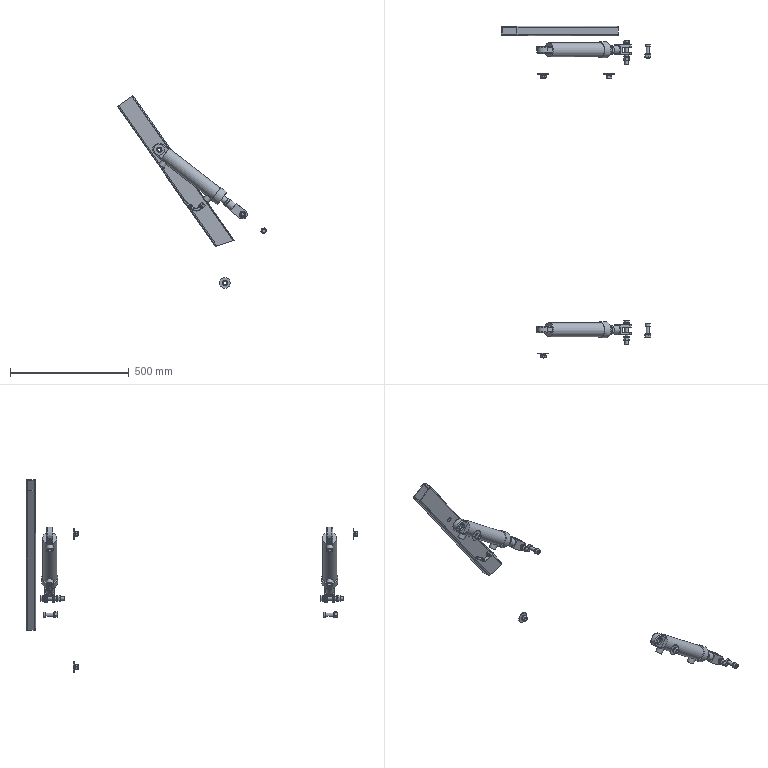Part | STEP file | COMPOUND | 36 solids | 457 faces | box 628.615 x 1399 x 812.176 mm | volume 2722476 mm3 | plane 261 | cylinder 124 | cone 37 | other 29 | torus 6 | commonest cylinder face diameters 28 x12 6 x8 8 x8 14 x7 14.001 x7 14.55 x7